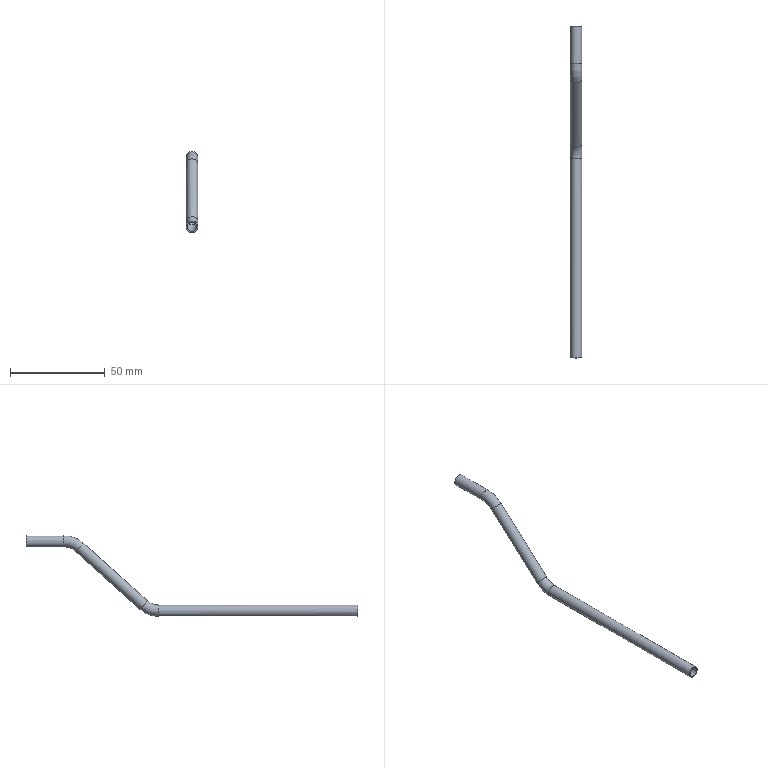Part | STEP file | 1-51.6 | 1 solid | 12 faces | box 6 x 175 x 42.678 mm | volume 1626 mm3 | cylinder 6 | torus 4 | plane 2 | commonest cylinder face diameters 5 x3 6 x3
STEP:
#1=CARTESIAN_POINT('',(0.,0.,0.));
#2=DIRECTION('',(0.,0.,1.));
#3=DIRECTION('',(1.,0.,0.));
#4=AXIS2_PLACEMENT_3D('',#1,#2,#3);
#5=CARTESIAN_POINT('',(3.,0.,0.));
#6=VERTEX_POINT('',#5);
#7=CARTESIAN_POINT('',(0.,0.,0.));
#8=DIRECTION('',(0.,-1.,0.));
#9=DIRECTION('',(1.,0.,0.));
#10=AXIS2_PLACEMENT_3D('',#7,#8,#9);
#11=CIRCLE('',#10,3.);
#12=CARTESIAN_POINT('',(0.,0.,0.));
#13=DIRECTION('',(0.,1.,0.));
#14=DIRECTION('',(1.,0.,0.));
#15=AXIS2_PLACEMENT_3D('',#12,#13,#14);
#16=CYLINDRICAL_SURFACE('',#15,3.);
#17=CARTESIAN_POINT('',(6.283,0.));
#18=DIRECTION('',(-1.,0.));
#19=VECTOR('',#18,1.);
#20=LINE('',#17,#19);
#21=(GEOMETRIC_REPRESENTATION_CONTEXT(2)PARAMETRIC_REPRESENTATION_CONTEXT()REPRESENTATION_CONTEXT('',''));
#22=DEFINITIONAL_REPRESENTATION('',(#20),#21);
#23=PCURVE('',#16,#22);
#24=CARTESIAN_POINT('',(0.,0.,0.));
#25=DIRECTION('',(0.,-1.,0.));
#26=DIRECTION('',(0.,0.,-1.));
#27=AXIS2_PLACEMENT_3D('',#24,#25,#26);
#28=PLANE('',#27);
#29=CARTESIAN_POINT('',(0.,0.));
#30=DIRECTION('',(0.,1.));
#31=AXIS2_PLACEMENT_2D('',#29,#30);
#32=CIRCLE('',#31,3.);
#33=(GEOMETRIC_REPRESENTATION_CONTEXT(2)PARAMETRIC_REPRESENTATION_CONTEXT()REPRESENTATION_CONTEXT('',''));
#34=DEFINITIONAL_REPRESENTATION('',(#32),#33);
#35=PCURVE('',#28,#34);
#36=SURFACE_CURVE('',#11,(#23,#35),.PCURVE_S1.);
#37=EDGE_CURVE('',#6,#6,#36,.T.);
#38=ORIENTED_EDGE('',*,*,#37,.F.);
#39=CARTESIAN_POINT('',(3.,105.,0.));
#40=VERTEX_POINT('',#39);
#41=CARTESIAN_POINT('',(3.,0.,0.));
#42=DIRECTION('',(0.,1.,0.));
#43=VECTOR('',#42,1.);
#44=LINE('',#41,#43);
#45=CARTESIAN_POINT('',(6.283,0.));
#46=DIRECTION('',(0.,1.));
#47=VECTOR('',#46,1.);
#48=LINE('',#45,#47);
#49=(GEOMETRIC_REPRESENTATION_CONTEXT(2)PARAMETRIC_REPRESENTATION_CONTEXT()REPRESENTATION_CONTEXT('',''));
#50=DEFINITIONAL_REPRESENTATION('',(#48),#49);
#51=PCURVE('',#16,#50);
#52=CARTESIAN_POINT('',(0.,0.));
#53=DIRECTION('',(0.,1.));
#54=VECTOR('',#53,1.);
#55=LINE('',#52,#54);
#56=(GEOMETRIC_REPRESENTATION_CONTEXT(2)PARAMETRIC_REPRESENTATION_CONTEXT()REPRESENTATION_CONTEXT('',''));
#57=DEFINITIONAL_REPRESENTATION('',(#55),#56);
#58=PCURVE('',#16,#57);
#59=SEAM_CURVE('',#44,(#51,#58),.PCURVE_S1.);
#60=EDGE_CURVE('',#6,#40,#59,.T.);
#61=ORIENTED_EDGE('',*,*,#60,.T.);
#62=CARTESIAN_POINT('',(0.,105.,-3.));
#63=VERTEX_POINT('',#62);
#64=CARTESIAN_POINT('',(0.,105.,0.));
#65=DIRECTION('',(0.,1.,0.));
#66=DIRECTION('',(0.,0.,-1.));
#67=AXIS2_PLACEMENT_3D('',#64,#65,#66);
#68=CIRCLE('',#67,3.);
#69=CARTESIAN_POINT('',(1.571,105.));
#70=DIRECTION('',(1.,0.));
#71=VECTOR('',#70,1.);
#72=LINE('',#69,#71);
#73=(GEOMETRIC_REPRESENTATION_CONTEXT(2)PARAMETRIC_REPRESENTATION_CONTEXT()REPRESENTATION_CONTEXT('',''));
#74=DEFINITIONAL_REPRESENTATION('',(#72),#73);
#75=PCURVE('',#16,#74);
#76=CARTESIAN_POINT('',(0.,105.,12.));
#77=DIRECTION('',(-1.,0.,0.));
#78=DIRECTION('',(0.,0.,-1.));
#79=AXIS2_PLACEMENT_3D('',#76,#77,#78);
#80=TOROIDAL_SURFACE('',#79,12.,3.);
#81=CARTESIAN_POINT('',(6.283,0.));
#82=DIRECTION('',(0.,1.));
#83=VECTOR('',#82,1.);
#84=LINE('',#81,#83);
#85=(GEOMETRIC_REPRESENTATION_CONTEXT(2)PARAMETRIC_REPRESENTATION_CONTEXT()REPRESENTATION_CONTEXT('',''));
#86=DEFINITIONAL_REPRESENTATION('',(#84),#85);
#87=PCURVE('',#80,#86);
#88=SURFACE_CURVE('',#68,(#75,#87),.PCURVE_S1.);
#89=EDGE_CURVE('',#63,#40,#88,.T.);
#90=ORIENTED_EDGE('',*,*,#89,.F.);
#91=CARTESIAN_POINT('',(0.,105.,0.));
#92=DIRECTION('',(0.,1.,0.));
#93=DIRECTION('',(1.,0.,0.));
#94=AXIS2_PLACEMENT_3D('',#91,#92,#93);
#95=CIRCLE('',#94,3.);
#96=CARTESIAN_POINT('',(0.,105.));
#97=DIRECTION('',(1.,0.));
#98=VECTOR('',#97,1.);
#99=LINE('',#96,#98);
#100=(GEOMETRIC_REPRESENTATION_CONTEXT(2)PARAMETRIC_REPRESENTATION_CONTEXT()REPRESENTATION_CONTEXT('',''));
#101=DEFINITIONAL_REPRESENTATION('',(#99),#100);
#102=PCURVE('',#16,#101);
#103=CARTESIAN_POINT('',(6.283,4.712));
#104=DIRECTION('',(0.,1.));
#105=VECTOR('',#104,1.);
#106=LINE('',#103,#105);
#107=(GEOMETRIC_REPRESENTATION_CONTEXT(2)PARAMETRIC_REPRESENTATION_CONTEXT()REPRESENTATION_CONTEXT('',''));
#108=DEFINITIONAL_REPRESENTATION('',(#106),#107);
#109=PCURVE('',#80,#108);
#110=SURFACE_CURVE('',#95,(#102,#109),.PCURVE_S1.);
#111=EDGE_CURVE('',#40,#63,#110,.T.);
#112=ORIENTED_EDGE('',*,*,#111,.F.);
#113=ORIENTED_EDGE('',*,*,#60,.F.);
#114=EDGE_LOOP('',(#38,#61,#90,#112,#113));
#115=FACE_BOUND('',#114,.T.);
#116=ADVANCED_FACE('',(#115),#16,.T.);
#117=ORIENTED_EDGE('',*,*,#89,.T.);
#118=ORIENTED_EDGE('',*,*,#111,.T.);
#119=CARTESIAN_POINT('',(0.,115.028,0.8451));
#120=VERTEX_POINT('',#119);
#121=CARTESIAN_POINT('',(0.,105.,12.));
#122=DIRECTION('',(1.,0.,0.));
#123=DIRECTION('',(0.,0.,-1.));
#124=AXIS2_PLACEMENT_3D('',#121,#122,#123);
#125=CIRCLE('',#124,15.);
#126=CARTESIAN_POINT('',(6.283,6.283));
#127=DIRECTION('',(-1.,0.));
#128=VECTOR('',#127,1.);
#129=LINE('',#126,#128);
#130=(GEOMETRIC_REPRESENTATION_CONTEXT(2)PARAMETRIC_REPRESENTATION_CONTEXT()REPRESENTATION_CONTEXT('',''));
#131=DEFINITIONAL_REPRESENTATION('',(#129),#130);
#132=PCURVE('',#80,#131);
#133=CARTESIAN_POINT('',(6.283,0.));
#134=DIRECTION('',(-1.,0.));
#135=VECTOR('',#134,1.);
#136=LINE('',#133,#135);
#137=(GEOMETRIC_REPRESENTATION_CONTEXT(2)PARAMETRIC_REPRESENTATION_CONTEXT()REPRESENTATION_CONTEXT('',''));
#138=DEFINITIONAL_REPRESENTATION('',(#136),#137);
#139=PCURVE('',#80,#138);
#140=SEAM_CURVE('',#125,(#132,#139),.PCURVE_S1.);
#141=EDGE_CURVE('',#63,#120,#140,.T.);
#142=ORIENTED_EDGE('',*,*,#141,.T.);
#143=CARTESIAN_POINT('',(3.,113.023,3.076));
#144=VERTEX_POINT('',#143);
#145=CARTESIAN_POINT('',(0.,113.023,3.076));
#146=DIRECTION('',(0.,-0.7437,-0.6686));
#147=DIRECTION('',(0.,0.6686,-0.7437));
#148=AXIS2_PLACEMENT_3D('',#145,#146,#147);
#149=CIRCLE('',#148,3.);
#150=CARTESIAN_POINT('',(5.551,6.283));
#151=DIRECTION('',(0.,-1.));
#152=VECTOR('',#151,1.);
#153=LINE('',#150,#152);
#154=(GEOMETRIC_REPRESENTATION_CONTEXT(2)PARAMETRIC_REPRESENTATION_CONTEXT()REPRESENTATION_CONTEXT('',''));
#155=DEFINITIONAL_REPRESENTATION('',(#153),#154);
#156=PCURVE('',#80,#155);
#157=CARTESIAN_POINT('',(0.,113.023,3.076));
#158=DIRECTION('',(0.,0.7437,0.6686));
#159=DIRECTION('',(1.,0.,0.));
#160=AXIS2_PLACEMENT_3D('',#157,#158,#159);
#161=CYLINDRICAL_SURFACE('',#160,3.);
#162=CARTESIAN_POINT('',(1.571,0.));
#163=DIRECTION('',(-1.,0.));
#164=VECTOR('',#163,1.);
#165=LINE('',#162,#164);
#166=(GEOMETRIC_REPRESENTATION_CONTEXT(2)PARAMETRIC_REPRESENTATION_CONTEXT()REPRESENTATION_CONTEXT('',''));
#167=DEFINITIONAL_REPRESENTATION('',(#165),#166);
#168=PCURVE('',#161,#167);
#169=SURFACE_CURVE('',#149,(#156,#168),.PCURVE_S1.);
#170=EDGE_CURVE('',#120,#144,#169,.T.);
#171=ORIENTED_EDGE('',*,*,#170,.T.);
#172=CARTESIAN_POINT('',(0.,113.023,3.076));
#173=DIRECTION('',(0.,-0.7437,-0.6686));
#174=DIRECTION('',(1.,0.,0.));
#175=AXIS2_PLACEMENT_3D('',#172,#173,#174);
#176=CIRCLE('',#175,3.);
#177=CARTESIAN_POINT('',(5.551,4.712));
#178=DIRECTION('',(0.,-1.));
#179=VECTOR('',#178,1.);
#180=LINE('',#177,#179);
#181=(GEOMETRIC_REPRESENTATION_CONTEXT(2)PARAMETRIC_REPRESENTATION_CONTEXT()REPRESENTATION_CONTEXT('',''));
#182=DEFINITIONAL_REPRESENTATION('',(#180),#181);
#183=PCURVE('',#80,#182);
#184=CARTESIAN_POINT('',(6.283,0.));
#185=DIRECTION('',(-1.,0.));
#186=VECTOR('',#185,1.);
#187=LINE('',#184,#186);
#188=(GEOMETRIC_REPRESENTATION_CONTEXT(2)PARAMETRIC_REPRESENTATION_CONTEXT()REPRESENTATION_CONTEXT('',''));
#189=DEFINITIONAL_REPRESENTATION('',(#187),#188);
#190=PCURVE('',#161,#189);
#191=SURFACE_CURVE('',#176,(#183,#190),.PCURVE_S1.);
#192=EDGE_CURVE('',#144,#120,#191,.T.);
#193=ORIENTED_EDGE('',*,*,#192,.T.);
#194=ORIENTED_EDGE('',*,*,#141,.F.);
#195=EDGE_LOOP('',(#117,#118,#142,#171,#193,#194));
#196=FACE_BOUND('',#195,.T.);
#197=ADVANCED_FACE('',(#196),#80,.T.);
#198=ORIENTED_EDGE('',*,*,#170,.F.);
#199=ORIENTED_EDGE('',*,*,#192,.F.);
#200=CARTESIAN_POINT('',(3.,146.977,33.602));
#201=VERTEX_POINT('',#200);
#202=CARTESIAN_POINT('',(3.,113.023,3.076));
#203=DIRECTION('',(0.,0.7437,0.6686));
#204=VECTOR('',#203,1.);
#205=LINE('',#202,#204);
#206=CARTESIAN_POINT('',(6.283,0.));
#207=DIRECTION('',(0.,1.));
#208=VECTOR('',#207,1.);
#209=LINE('',#206,#208);
#210=(GEOMETRIC_REPRESENTATION_CONTEXT(2)PARAMETRIC_REPRESENTATION_CONTEXT()REPRESENTATION_CONTEXT('',''));
#211=DEFINITIONAL_REPRESENTATION('',(#209),#210);
#212=PCURVE('',#161,#211);
#213=CARTESIAN_POINT('',(0.,0.));
#214=DIRECTION('',(0.,1.));
#215=VECTOR('',#214,1.);
#216=LINE('',#213,#215);
#217=(GEOMETRIC_REPRESENTATION_CONTEXT(2)PARAMETRIC_REPRESENTATION_CONTEXT()REPRESENTATION_CONTEXT('',''));
#218=DEFINITIONAL_REPRESENTATION('',(#216),#217);
#219=PCURVE('',#161,#218);
#220=SEAM_CURVE('',#205,(#212,#219),.PCURVE_S1.);
#221=EDGE_CURVE('',#144,#201,#220,.T.);
#222=ORIENTED_EDGE('',*,*,#221,.T.);
#223=CARTESIAN_POINT('',(-3.,146.977,33.602));
#224=VERTEX_POINT('',#223);
#225=CARTESIAN_POINT('',(0.,146.977,33.602));
#226=DIRECTION('',(0.,0.7437,0.6686));
#227=DIRECTION('',(-1.,0.,0.));
#228=AXIS2_PLACEMENT_3D('',#225,#226,#227);
#229=CIRCLE('',#228,3.);
#230=CARTESIAN_POINT('',(3.142,45.659));
#231=DIRECTION('',(1.,0.));
#232=VECTOR('',#231,1.);
#233=LINE('',#230,#232);
#234=(GEOMETRIC_REPRESENTATION_CONTEXT(2)PARAMETRIC_REPRESENTATION_CONTEXT()REPRESENTATION_CONTEXT('',''));
#235=DEFINITIONAL_REPRESENTATION('',(#233),#234);
#236=PCURVE('',#161,#235);
#237=CARTESIAN_POINT('',(0.,155.,24.678));
#238=DIRECTION('',(1.,0.,0.));
#239=DIRECTION('',(0.,-0.6686,0.7437));
#240=AXIS2_PLACEMENT_3D('',#237,#238,#239);
#241=TOROIDAL_SURFACE('',#240,12.,3.);
#242=CARTESIAN_POINT('',(6.283,-1.571));
#243=DIRECTION('',(0.,1.));
#244=VECTOR('',#243,1.);
#245=LINE('',#242,#244);
#246=(GEOMETRIC_REPRESENTATION_CONTEXT(2)PARAMETRIC_REPRESENTATION_CONTEXT()REPRESENTATION_CONTEXT('',''));
#247=DEFINITIONAL_REPRESENTATION('',(#245),#246);
#248=PCURVE('',#241,#247);
#249=SURFACE_CURVE('',#229,(#236,#248),.PCURVE_S1.);
#250=EDGE_CURVE('',#224,#201,#249,.T.);
#251=ORIENTED_EDGE('',*,*,#250,.F.);
#252=CARTESIAN_POINT('',(0.,146.977,33.602));
#253=DIRECTION('',(0.,0.7437,0.6686));
#254=DIRECTION('',(1.,0.,0.));
#255=AXIS2_PLACEMENT_3D('',#252,#253,#254);
#256=CIRCLE('',#255,3.);
#257=CARTESIAN_POINT('',(0.,45.659));
#258=DIRECTION('',(1.,0.));
#259=VECTOR('',#258,1.);
#260=LINE('',#257,#259);
#261=(GEOMETRIC_REPRESENTATION_CONTEXT(2)PARAMETRIC_REPRESENTATION_CONTEXT()REPRESENTATION_CONTEXT('',''));
#262=DEFINITIONAL_REPRESENTATION('',(#260),#261);
#263=PCURVE('',#161,#262);
#264=CARTESIAN_POINT('',(6.283,1.571));
#265=DIRECTION('',(0.,1.));
#266=VECTOR('',#265,1.);
#267=LINE('',#264,#266);
#268=(GEOMETRIC_REPRESENTATION_CONTEXT(2)PARAMETRIC_REPRESENTATION_CONTEXT()REPRESENTATION_CONTEXT('',''));
#269=DEFINITIONAL_REPRESENTATION('',(#267),#268);
#270=PCURVE('',#241,#269);
#271=SURFACE_CURVE('',#256,(#263,#270),.PCURVE_S1.);
#272=EDGE_CURVE('',#201,#224,#271,.T.);
#273=ORIENTED_EDGE('',*,*,#272,.F.);
#274=ORIENTED_EDGE('',*,*,#221,.F.);
#275=EDGE_LOOP('',(#198,#199,#222,#251,#273,#274));
#276=FACE_BOUND('',#275,.T.);
#277=ADVANCED_FACE('',(#276),#161,.T.);
#278=ORIENTED_EDGE('',*,*,#250,.T.);
#279=ORIENTED_EDGE('',*,*,#272,.T.);
#280=CARTESIAN_POINT('',(-3.,155.,36.678));
#281=VERTEX_POINT('',#280);
#282=CARTESIAN_POINT('',(-3.,155.,24.678));
#283=DIRECTION('',(-1.,0.,0.));
#284=DIRECTION('',(0.,-0.6686,0.7437));
#285=AXIS2_PLACEMENT_3D('',#282,#283,#284);
#286=CIRCLE('',#285,12.);
#287=CARTESIAN_POINT('',(6.283,4.712));
#288=DIRECTION('',(-1.,0.));
#289=VECTOR('',#288,1.);
#290=LINE('',#287,#289);
#291=(GEOMETRIC_REPRESENTATION_CONTEXT(2)PARAMETRIC_REPRESENTATION_CONTEXT()REPRESENTATION_CONTEXT('',''));
#292=DEFINITIONAL_REPRESENTATION('',(#290),#291);
#293=PCURVE('',#241,#292);
#294=CARTESIAN_POINT('',(6.283,-1.571));
#295=DIRECTION('',(-1.,0.));
#296=VECTOR('',#295,1.);
#297=LINE('',#294,#296);
#298=(GEOMETRIC_REPRESENTATION_CONTEXT(2)PARAMETRIC_REPRESENTATION_CONTEXT()REPRESENTATION_CONTEXT('',''));
#299=DEFINITIONAL_REPRESENTATION('',(#297),#298);
#300=PCURVE('',#241,#299);
#301=SEAM_CURVE('',#286,(#293,#300),.PCURVE_S1.);
#302=EDGE_CURVE('',#224,#281,#301,.T.);
#303=ORIENTED_EDGE('',*,*,#302,.T.);
#304=CARTESIAN_POINT('',(3.,155.,36.678));
#305=VERTEX_POINT('',#304);
#306=CARTESIAN_POINT('',(0.,155.,36.678));
#307=DIRECTION('',(0.,-1.,0.));
#308=DIRECTION('',(-1.,0.,0.));
#309=AXIS2_PLACEMENT_3D('',#306,#307,#308);
#310=CIRCLE('',#309,3.);
#311=CARTESIAN_POINT('',(5.551,4.712));
#312=DIRECTION('',(0.,-1.));
#313=VECTOR('',#312,1.);
#314=LINE('',#311,#313);
#315=(GEOMETRIC_REPRESENTATION_CONTEXT(2)PARAMETRIC_REPRESENTATION_CONTEXT()REPRESENTATION_CONTEXT('',''));
#316=DEFINITIONAL_REPRESENTATION('',(#314),#315);
#317=PCURVE('',#241,#316);
#318=CARTESIAN_POINT('',(0.,155.,36.678));
#319=DIRECTION('',(0.,1.,0.));
#320=DIRECTION('',(1.,0.,0.));
#321=AXIS2_PLACEMENT_3D('',#318,#319,#320);
#322=CYLINDRICAL_SURFACE('',#321,3.);
#323=CARTESIAN_POINT('',(3.142,0.));
#324=DIRECTION('',(-1.,0.));
#325=VECTOR('',#324,1.);
#326=LINE('',#323,#325);
#327=(GEOMETRIC_REPRESENTATION_CONTEXT(2)PARAMETRIC_REPRESENTATION_CONTEXT()REPRESENTATION_CONTEXT('',''));
#328=DEFINITIONAL_REPRESENTATION('',(#326),#327);
#329=PCURVE('',#322,#328);
#330=SURFACE_CURVE('',#310,(#317,#329),.PCURVE_S1.);
#331=EDGE_CURVE('',#281,#305,#330,.T.);
#332=ORIENTED_EDGE('',*,*,#331,.T.);
#333=CARTESIAN_POINT('',(0.,155.,36.678));
#334=DIRECTION('',(0.,-1.,0.));
#335=DIRECTION('',(1.,0.,0.));
#336=AXIS2_PLACEMENT_3D('',#333,#334,#335);
#337=CIRCLE('',#336,3.);
#338=CARTESIAN_POINT('',(5.551,1.571));
#339=DIRECTION('',(0.,-1.));
#340=VECTOR('',#339,1.);
#341=LINE('',#338,#340);
#342=(GEOMETRIC_REPRESENTATION_CONTEXT(2)PARAMETRIC_REPRESENTATION_CONTEXT()REPRESENTATION_CONTEXT('',''));
#343=DEFINITIONAL_REPRESENTATION('',(#341),#342);
#344=PCURVE('',#241,#343);
#345=CARTESIAN_POINT('',(6.283,0.));
#346=DIRECTION('',(-1.,0.));
#347=VECTOR('',#346,1.);
#348=LINE('',#345,#347);
#349=(GEOMETRIC_REPRESENTATION_CONTEXT(2)PARAMETRIC_REPRESENTATION_CONTEXT()REPRESENTATION_CONTEXT('',''));
#350=DEFINITIONAL_REPRESENTATION('',(#348),#349);
#351=PCURVE('',#322,#350);
#352=SURFACE_CURVE('',#337,(#344,#351),.PCURVE_S1.);
#353=EDGE_CURVE('',#305,#281,#352,.T.);
#354=ORIENTED_EDGE('',*,*,#353,.T.);
#355=ORIENTED_EDGE('',*,*,#302,.F.);
#356=EDGE_LOOP('',(#278,#279,#303,#332,#354,#355));
#357=FACE_BOUND('',#356,.T.);
#358=ADVANCED_FACE('',(#357),#241,.T.);
#359=ORIENTED_EDGE('',*,*,#331,.F.);
#360=ORIENTED_EDGE('',*,*,#353,.F.);
#361=CARTESIAN_POINT('',(3.,175.,36.678));
#362=VERTEX_POINT('',#361);
#363=CARTESIAN_POINT('',(3.,155.,36.678));
#364=DIRECTION('',(0.,1.,0.));
#365=VECTOR('',#364,1.);
#366=LINE('',#363,#365);
#367=CARTESIAN_POINT('',(6.283,0.));
#368=DIRECTION('',(0.,1.));
#369=VECTOR('',#368,1.);
#370=LINE('',#367,#369);
#371=(GEOMETRIC_REPRESENTATION_CONTEXT(2)PARAMETRIC_REPRESENTATION_CONTEXT()REPRESENTATION_CONTEXT('',''));
#372=DEFINITIONAL_REPRESENTATION('',(#370),#371);
#373=PCURVE('',#322,#372);
#374=CARTESIAN_POINT('',(0.,0.));
#375=DIRECTION('',(0.,1.));
#376=VECTOR('',#375,1.);
#377=LINE('',#374,#376);
#378=(GEOMETRIC_REPRESENTATION_CONTEXT(2)PARAMETRIC_REPRESENTATION_CONTEXT()REPRESENTATION_CONTEXT('',''));
#379=DEFINITIONAL_REPRESENTATION('',(#377),#378);
#380=PCURVE('',#322,#379);
#381=SEAM_CURVE('',#366,(#373,#380),.PCURVE_S1.);
#382=EDGE_CURVE('',#305,#362,#381,.T.);
#383=ORIENTED_EDGE('',*,*,#382,.T.);
#384=CARTESIAN_POINT('',(0.,175.,36.678));
#385=DIRECTION('',(0.,1.,0.));
#386=DIRECTION('',(1.,0.,0.));
#387=AXIS2_PLACEMENT_3D('',#384,#385,#386);
#388=CIRCLE('',#387,3.);
#389=CARTESIAN_POINT('',(0.,20.));
#390=DIRECTION('',(1.,0.));
#391=VECTOR('',#390,1.);
#392=LINE('',#389,#391);
#393=(GEOMETRIC_REPRESENTATION_CONTEXT(2)PARAMETRIC_REPRESENTATION_CONTEXT()REPRESENTATION_CONTEXT('',''));
#394=DEFINITIONAL_REPRESENTATION('',(#392),#393);
#395=PCURVE('',#322,#394);
#396=CARTESIAN_POINT('',(0.,175.,36.678));
#397=DIRECTION('',(0.,1.,0.));
#398=DIRECTION('',(0.,0.,1.));
#399=AXIS2_PLACEMENT_3D('',#396,#397,#398);
#400=PLANE('',#399);
#401=CARTESIAN_POINT('',(0.,0.));
#402=DIRECTION('',(0.,1.));
#403=AXIS2_PLACEMENT_2D('',#401,#402);
#404=CIRCLE('',#403,3.);
#405=(GEOMETRIC_REPRESENTATION_CONTEXT(2)PARAMETRIC_REPRESENTATION_CONTEXT()REPRESENTATION_CONTEXT('',''));
#406=DEFINITIONAL_REPRESENTATION('',(#404),#405);
#407=PCURVE('',#400,#406);
#408=SURFACE_CURVE('',#388,(#395,#407),.PCURVE_S1.);
#409=EDGE_CURVE('',#362,#362,#408,.T.);
#410=ORIENTED_EDGE('',*,*,#409,.F.);
#411=ORIENTED_EDGE('',*,*,#382,.F.);
#412=EDGE_LOOP('',(#359,#360,#383,#410,#411));
#413=FACE_BOUND('',#412,.T.);
#414=ADVANCED_FACE('',(#413),#322,.T.);
#415=ORIENTED_EDGE('',*,*,#37,.T.);
#416=EDGE_LOOP('',(#415));
#417=FACE_BOUND('',#416,.T.);
#418=CARTESIAN_POINT('',(2.5,0.,0.));
#419=VERTEX_POINT('',#418);
#420=CARTESIAN_POINT('',(0.,0.,0.));
#421=DIRECTION('',(0.,-1.,0.));
#422=DIRECTION('',(1.,0.,0.));
#423=AXIS2_PLACEMENT_3D('',#420,#421,#422);
#424=CIRCLE('',#423,2.5);
#425=CARTESIAN_POINT('',(0.,0.));
#426=DIRECTION('',(0.,1.));
#427=AXIS2_PLACEMENT_2D('',#425,#426);
#428=CIRCLE('',#427,2.5);
#429=(GEOMETRIC_REPRESENTATION_CONTEXT(2)PARAMETRIC_REPRESENTATION_CONTEXT()REPRESENTATION_CONTEXT('',''));
#430=DEFINITIONAL_REPRESENTATION('',(#428),#429);
#431=PCURVE('',#28,#430);
#432=CARTESIAN_POINT('',(0.,0.,0.));
#433=DIRECTION('',(0.,1.,0.));
#434=DIRECTION('',(1.,0.,0.));
#435=AXIS2_PLACEMENT_3D('',#432,#433,#434);
#436=CYLINDRICAL_SURFACE('',#435,2.5);
#437=CARTESIAN_POINT('',(6.283,0.));
#438=DIRECTION('',(-1.,0.));
#439=VECTOR('',#438,1.);
#440=LINE('',#437,#439);
#441=(GEOMETRIC_REPRESENTATION_CONTEXT(2)PARAMETRIC_REPRESENTATION_CONTEXT()REPRESENTATION_CONTEXT('',''));
#442=DEFINITIONAL_REPRESENTATION('',(#440),#441);
#443=PCURVE('',#436,#442);
#444=SURFACE_CURVE('',#424,(#431,#443),.PCURVE_S1.);
#445=EDGE_CURVE('',#419,#419,#444,.T.);
#446=ORIENTED_EDGE('',*,*,#445,.F.);
#447=EDGE_LOOP('',(#446));
#448=FACE_BOUND('',#447,.T.);
#449=ADVANCED_FACE('',(#417,#448),#28,.T.);
#450=ORIENTED_EDGE('',*,*,#409,.T.);
#451=EDGE_LOOP('',(#450));
#452=FACE_BOUND('',#451,.T.);
#453=CARTESIAN_POINT('',(2.5,175.,36.678));
#454=VERTEX_POINT('',#453);
#455=CARTESIAN_POINT('',(0.,175.,36.678));
#456=DIRECTION('',(0.,1.,0.));
#457=DIRECTION('',(1.,0.,0.));
#458=AXIS2_PLACEMENT_3D('',#455,#456,#457);
#459=CIRCLE('',#458,2.5);
#460=CARTESIAN_POINT('',(0.,0.));
#461=DIRECTION('',(0.,1.));
#462=AXIS2_PLACEMENT_2D('',#460,#461);
#463=CIRCLE('',#462,2.5);
#464=(GEOMETRIC_REPRESENTATION_CONTEXT(2)PARAMETRIC_REPRESENTATION_CONTEXT()REPRESENTATION_CONTEXT('',''));
#465=DEFINITIONAL_REPRESENTATION('',(#463),#464);
#466=PCURVE('',#400,#465);
#467=CARTESIAN_POINT('',(0.,155.,36.678));
#468=DIRECTION('',(0.,1.,0.));
#469=DIRECTION('',(1.,0.,0.));
#470=AXIS2_PLACEMENT_3D('',#467,#468,#469);
#471=CYLINDRICAL_SURFACE('',#470,2.5);
#472=CARTESIAN_POINT('',(0.,20.));
#473=DIRECTION('',(1.,0.));
#474=VECTOR('',#473,1.);
#475=LINE('',#472,#474);
#476=(GEOMETRIC_REPRESENTATION_CONTEXT(2)PARAMETRIC_REPRESENTATION_CONTEXT()REPRESENTATION_CONTEXT('',''));
#477=DEFINITIONAL_REPRESENTATION('',(#475),#476);
#478=PCURVE('',#471,#477);
#479=SURFACE_CURVE('',#459,(#466,#478),.PCURVE_S1.);
#480=EDGE_CURVE('',#454,#454,#479,.T.);
#481=ORIENTED_EDGE('',*,*,#480,.F.);
#482=EDGE_LOOP('',(#481));
#483=FACE_BOUND('',#482,.T.);
#484=ADVANCED_FACE('',(#452,#483),#400,.T.);
#485=ORIENTED_EDGE('',*,*,#445,.F.);
#486=CARTESIAN_POINT('',(2.5,105.,0.));
#487=VERTEX_POINT('',#486);
#488=CARTESIAN_POINT('',(2.5,0.,0.));
#489=DIRECTION('',(0.,1.,0.));
#490=VECTOR('',#489,1.);
#491=LINE('',#488,#490);
#492=CARTESIAN_POINT('',(6.283,0.));
#493=DIRECTION('',(0.,1.));
#494=VECTOR('',#493,1.);
#495=LINE('',#492,#494);
#496=(GEOMETRIC_REPRESENTATION_CONTEXT(2)PARAMETRIC_REPRESENTATION_CONTEXT()REPRESENTATION_CONTEXT('',''));
#497=DEFINITIONAL_REPRESENTATION('',(#495),#496);
#498=PCURVE('',#436,#497);
#499=CARTESIAN_POINT('',(0.,0.));
#500=DIRECTION('',(0.,1.));
#501=VECTOR('',#500,1.);
#502=LINE('',#499,#501);
#503=(GEOMETRIC_REPRESENTATION_CONTEXT(2)PARAMETRIC_REPRESENTATION_CONTEXT()REPRESENTATION_CONTEXT('',''));
#504=DEFINITIONAL_REPRESENTATION('',(#502),#503);
#505=PCURVE('',#436,#504);
#506=SEAM_CURVE('',#491,(#498,#505),.PCURVE_S1.);
#507=EDGE_CURVE('',#419,#487,#506,.T.);
#508=ORIENTED_EDGE('',*,*,#507,.T.);
#509=CARTESIAN_POINT('',(0.,105.,-2.5));
#510=VERTEX_POINT('',#509);
#511=CARTESIAN_POINT('',(0.,105.,0.));
#512=DIRECTION('',(0.,1.,0.));
#513=DIRECTION('',(0.,0.,-1.));
#514=AXIS2_PLACEMENT_3D('',#511,#512,#513);
#515=CIRCLE('',#514,2.5);
#516=CARTESIAN_POINT('',(1.571,105.));
#517=DIRECTION('',(1.,0.));
#518=VECTOR('',#517,1.);
#519=LINE('',#516,#518);
#520=(GEOMETRIC_REPRESENTATION_CONTEXT(2)PARAMETRIC_REPRESENTATION_CONTEXT()REPRESENTATION_CONTEXT('',''));
#521=DEFINITIONAL_REPRESENTATION('',(#519),#520);
#522=PCURVE('',#436,#521);
#523=CARTESIAN_POINT('',(0.,105.,12.));
#524=DIRECTION('',(-1.,0.,0.));
#525=DIRECTION('',(0.,0.,-1.));
#526=AXIS2_PLACEMENT_3D('',#523,#524,#525);
#527=TOROIDAL_SURFACE('',#526,12.,2.5);
#528=CARTESIAN_POINT('',(6.283,0.));
#529=CARTESIAN_POINT('',(6.283,0.0714));
#530=CARTESIAN_POINT('',(6.283,0.2142));
#531=CARTESIAN_POINT('',(6.283,0.4284));
#532=CARTESIAN_POINT('',(6.283,0.6426));
#533=CARTESIAN_POINT('',(6.283,0.8568));
#534=CARTESIAN_POINT('',(6.283,1.071));
#535=CARTESIAN_POINT('',(6.283,1.285));
#536=CARTESIAN_POINT('',(6.283,1.499));
#537=CARTESIAN_POINT('',(6.283,1.714));
#538=CARTESIAN_POINT('',(6.283,1.928));
#539=CARTESIAN_POINT('',(6.283,2.142));
#540=CARTESIAN_POINT('',(6.283,2.356));
#541=CARTESIAN_POINT('',(6.283,2.57));
#542=CARTESIAN_POINT('',(6.283,2.785));
#543=CARTESIAN_POINT('',(6.283,2.999));
#544=CARTESIAN_POINT('',(6.283,3.213));
#545=CARTESIAN_POINT('',(6.283,3.427));
#546=CARTESIAN_POINT('',(6.283,3.641));
#547=CARTESIAN_POINT('',(6.283,3.856));
#548=CARTESIAN_POINT('',(6.283,4.07));
#549=CARTESIAN_POINT('',(6.283,4.284));
#550=CARTESIAN_POINT('',(6.283,4.498));
#551=CARTESIAN_POINT('',(6.283,4.641));
#552=CARTESIAN_POINT('',(6.283,4.712));
#553=B_SPLINE_CURVE_WITH_KNOTS('',3,(#528,#529,#530,#531,#532,#533,#534,#535,#536,#537,#538,#539,#540,#541,#542,#543,#544,#545,#546,#547,#548,#549,#550,#551,#552),.UNSPECIFIED.,.F.,.F.,(4,1,1,1,1,1,1,1,1,1,1,1,1,1,1,1,1,1,1,1,1,1,4),(0.,0.2142,0.4284,0.6426,0.8568,1.071,1.285,1.499,1.714,1.928,2.142,2.356,2.57,2.785,2.999,3.213,3.427,3.641,3.856,4.07,4.284,4.498,4.712),.QUASI_UNIFORM_KNOTS.);
#554=(GEOMETRIC_REPRESENTATION_CONTEXT(2)PARAMETRIC_REPRESENTATION_CONTEXT()REPRESENTATION_CONTEXT('',''));
#555=DEFINITIONAL_REPRESENTATION('',(#553),#554);
#556=PCURVE('',#527,#555);
#557=SURFACE_CURVE('',#515,(#522,#556),.PCURVE_S1.);
#558=EDGE_CURVE('',#510,#487,#557,.T.);
#559=ORIENTED_EDGE('',*,*,#558,.F.);
#560=CARTESIAN_POINT('',(0.,105.,0.));
#561=DIRECTION('',(0.,1.,0.));
#562=DIRECTION('',(1.,0.,0.));
#563=AXIS2_PLACEMENT_3D('',#560,#561,#562);
#564=CIRCLE('',#563,2.5);
#565=CARTESIAN_POINT('',(0.,105.));
#566=DIRECTION('',(1.,0.));
#567=VECTOR('',#566,1.);
#568=LINE('',#565,#567);
#569=(GEOMETRIC_REPRESENTATION_CONTEXT(2)PARAMETRIC_REPRESENTATION_CONTEXT()REPRESENTATION_CONTEXT('',''));
#570=DEFINITIONAL_REPRESENTATION('',(#568),#569);
#571=PCURVE('',#436,#570);
#572=CARTESIAN_POINT('',(6.283,4.712));
#573=DIRECTION('',(0.,1.));
#574=VECTOR('',#573,1.);
#575=LINE('',#572,#574);
#576=(GEOMETRIC_REPRESENTATION_CONTEXT(2)PARAMETRIC_REPRESENTATION_CONTEXT()REPRESENTATION_CONTEXT('',''));
#577=DEFINITIONAL_REPRESENTATION('',(#575),#576);
#578=PCURVE('',#527,#577);
#579=SURFACE_CURVE('',#564,(#571,#578),.PCURVE_S1.);
#580=EDGE_CURVE('',#487,#510,#579,.T.);
#581=ORIENTED_EDGE('',*,*,#580,.F.);
#582=ORIENTED_EDGE('',*,*,#507,.F.);
#583=EDGE_LOOP('',(#485,#508,#559,#581,#582));
#584=FACE_BOUND('',#583,.F.);
#585=ADVANCED_FACE('',(#584),#436,.F.);
#586=ORIENTED_EDGE('',*,*,#558,.T.);
#587=ORIENTED_EDGE('',*,*,#580,.T.);
#588=CARTESIAN_POINT('',(0.,114.694,1.217));
#589=VERTEX_POINT('',#588);
#590=CARTESIAN_POINT('',(0.,105.,12.));
#591=DIRECTION('',(1.,0.,0.));
#592=DIRECTION('',(0.,0.,-1.));
#593=AXIS2_PLACEMENT_3D('',#590,#591,#592);
#594=CIRCLE('',#593,14.5);
#595=CARTESIAN_POINT('',(6.283,6.283));
#596=DIRECTION('',(-1.,0.));
#597=VECTOR('',#596,1.);
#598=LINE('',#595,#597);
#599=(GEOMETRIC_REPRESENTATION_CONTEXT(2)PARAMETRIC_REPRESENTATION_CONTEXT()REPRESENTATION_CONTEXT('',''));
#600=DEFINITIONAL_REPRESENTATION('',(#598),#599);
#601=PCURVE('',#527,#600);
#602=CARTESIAN_POINT('',(6.283,0.));
#603=DIRECTION('',(-1.,0.));
#604=VECTOR('',#603,1.);
#605=LINE('',#602,#604);
#606=(GEOMETRIC_REPRESENTATION_CONTEXT(2)PARAMETRIC_REPRESENTATION_CONTEXT()REPRESENTATION_CONTEXT('',''));
#607=DEFINITIONAL_REPRESENTATION('',(#605),#606);
#608=PCURVE('',#527,#607);
#609=SEAM_CURVE('',#594,(#601,#608),.PCURVE_S1.);
#610=EDGE_CURVE('',#510,#589,#609,.T.);
#611=ORIENTED_EDGE('',*,*,#610,.T.);
#612=CARTESIAN_POINT('',(2.5,113.023,3.076));
#613=VERTEX_POINT('',#612);
#614=CARTESIAN_POINT('',(0.,113.023,3.076));
#615=DIRECTION('',(0.,-0.7437,-0.6686));
#616=DIRECTION('',(0.,0.6686,-0.7437));
#617=AXIS2_PLACEMENT_3D('',#614,#615,#616);
#618=CIRCLE('',#617,2.5);
#619=CARTESIAN_POINT('',(5.551,6.283));
#620=DIRECTION('',(0.,-1.));
#621=VECTOR('',#620,1.);
#622=LINE('',#619,#621);
#623=(GEOMETRIC_REPRESENTATION_CONTEXT(2)PARAMETRIC_REPRESENTATION_CONTEXT()REPRESENTATION_CONTEXT('',''));
#624=DEFINITIONAL_REPRESENTATION('',(#622),#623);
#625=PCURVE('',#527,#624);
#626=CARTESIAN_POINT('',(0.,113.023,3.076));
#627=DIRECTION('',(0.,0.7437,0.6686));
#628=DIRECTION('',(1.,0.,0.));
#629=AXIS2_PLACEMENT_3D('',#626,#627,#628);
#630=CYLINDRICAL_SURFACE('',#629,2.5);
#631=CARTESIAN_POINT('',(1.571,0.));
#632=DIRECTION('',(-1.,0.));
#633=VECTOR('',#632,1.);
#634=LINE('',#631,#633);
#635=(GEOMETRIC_REPRESENTATION_CONTEXT(2)PARAMETRIC_REPRESENTATION_CONTEXT()REPRESENTATION_CONTEXT('',''));
#636=DEFINITIONAL_REPRESENTATION('',(#634),#635);
#637=PCURVE('',#630,#636);
#638=SURFACE_CURVE('',#618,(#625,#637),.PCURVE_S1.);
#639=EDGE_CURVE('',#589,#613,#638,.T.);
#640=ORIENTED_EDGE('',*,*,#639,.T.);
#641=CARTESIAN_POINT('',(0.,113.023,3.076));
#642=DIRECTION('',(0.,-0.7437,-0.6686));
#643=DIRECTION('',(1.,0.,0.));
#644=AXIS2_PLACEMENT_3D('',#641,#642,#643);
#645=CIRCLE('',#644,2.5);
#646=CARTESIAN_POINT('',(5.551,4.712));
#647=DIRECTION('',(0.,-1.));
#648=VECTOR('',#647,1.);
#649=LINE('',#646,#648);
#650=(GEOMETRIC_REPRESENTATION_CONTEXT(2)PARAMETRIC_REPRESENTATION_CONTEXT()REPRESENTATION_CONTEXT('',''));
#651=DEFINITIONAL_REPRESENTATION('',(#649),#650);
#652=PCURVE('',#527,#651);
#653=CARTESIAN_POINT('',(6.283,0.));
#654=DIRECTION('',(-1.,0.));
#655=VECTOR('',#654,1.);
#656=LINE('',#653,#655);
#657=(GEOMETRIC_REPRESENTATION_CONTEXT(2)PARAMETRIC_REPRESENTATION_CONTEXT()REPRESENTATION_CONTEXT('',''));
#658=DEFINITIONAL_REPRESENTATION('',(#656),#657);
#659=PCURVE('',#630,#658);
#660=SURFACE_CURVE('',#645,(#652,#659),.PCURVE_S1.);
#661=EDGE_CURVE('',#613,#589,#660,.T.);
#662=ORIENTED_EDGE('',*,*,#661,.T.);
#663=ORIENTED_EDGE('',*,*,#610,.F.);
#664=EDGE_LOOP('',(#586,#587,#611,#640,#662,#663));
#665=FACE_BOUND('',#664,.F.);
#666=ADVANCED_FACE('',(#665),#527,.F.);
#667=ORIENTED_EDGE('',*,*,#639,.F.);
#668=ORIENTED_EDGE('',*,*,#661,.F.);
#669=CARTESIAN_POINT('',(2.5,146.977,33.602));
#670=VERTEX_POINT('',#669);
#671=CARTESIAN_POINT('',(2.5,113.023,3.076));
#672=DIRECTION('',(0.,0.7437,0.6686));
#673=VECTOR('',#672,1.);
#674=LINE('',#671,#673);
#675=CARTESIAN_POINT('',(6.283,0.));
#676=DIRECTION('',(0.,1.));
#677=VECTOR('',#676,1.);
#678=LINE('',#675,#677);
#679=(GEOMETRIC_REPRESENTATION_CONTEXT(2)PARAMETRIC_REPRESENTATION_CONTEXT()REPRESENTATION_CONTEXT('',''));
#680=DEFINITIONAL_REPRESENTATION('',(#678),#679);
#681=PCURVE('',#630,#680);
#682=CARTESIAN_POINT('',(0.,0.));
#683=DIRECTION('',(0.,1.));
#684=VECTOR('',#683,1.);
#685=LINE('',#682,#684);
#686=(GEOMETRIC_REPRESENTATION_CONTEXT(2)PARAMETRIC_REPRESENTATION_CONTEXT()REPRESENTATION_CONTEXT('',''));
#687=DEFINITIONAL_REPRESENTATION('',(#685),#686);
#688=PCURVE('',#630,#687);
#689=SEAM_CURVE('',#674,(#681,#688),.PCURVE_S1.);
#690=EDGE_CURVE('',#613,#670,#689,.T.);
#691=ORIENTED_EDGE('',*,*,#690,.T.);
#692=CARTESIAN_POINT('',(-2.5,146.977,33.602));
#693=VERTEX_POINT('',#692);
#694=CARTESIAN_POINT('',(0.,146.977,33.602));
#695=DIRECTION('',(0.,0.7437,0.6686));
#696=DIRECTION('',(-1.,0.,0.));
#697=AXIS2_PLACEMENT_3D('',#694,#695,#696);
#698=CIRCLE('',#697,2.5);
#699=CARTESIAN_POINT('',(3.142,45.659));
#700=DIRECTION('',(1.,0.));
#701=VECTOR('',#700,1.);
#702=LINE('',#699,#701);
#703=(GEOMETRIC_REPRESENTATION_CONTEXT(2)PARAMETRIC_REPRESENTATION_CONTEXT()REPRESENTATION_CONTEXT('',''));
#704=DEFINITIONAL_REPRESENTATION('',(#702),#703);
#705=PCURVE('',#630,#704);
#706=CARTESIAN_POINT('',(0.,155.,24.678));
#707=DIRECTION('',(1.,0.,0.));
#708=DIRECTION('',(0.,-0.6686,0.7437));
#709=AXIS2_PLACEMENT_3D('',#706,#707,#708);
#710=TOROIDAL_SURFACE('',#709,12.,2.5);
#711=CARTESIAN_POINT('',(6.283,-1.571));
#712=DIRECTION('',(0.,1.));
#713=VECTOR('',#712,1.);
#714=LINE('',#711,#713);
#715=(GEOMETRIC_REPRESENTATION_CONTEXT(2)PARAMETRIC_REPRESENTATION_CONTEXT()REPRESENTATION_CONTEXT('',''));
#716=DEFINITIONAL_REPRESENTATION('',(#714),#715);
#717=PCURVE('',#710,#716);
#718=SURFACE_CURVE('',#698,(#705,#717),.PCURVE_S1.);
#719=EDGE_CURVE('',#693,#670,#718,.T.);
#720=ORIENTED_EDGE('',*,*,#719,.F.);
#721=CARTESIAN_POINT('',(0.,146.977,33.602));
#722=DIRECTION('',(0.,0.7437,0.6686));
#723=DIRECTION('',(1.,0.,0.));
#724=AXIS2_PLACEMENT_3D('',#721,#722,#723);
#725=CIRCLE('',#724,2.5);
#726=CARTESIAN_POINT('',(0.,45.659));
#727=DIRECTION('',(1.,0.));
#728=VECTOR('',#727,1.);
#729=LINE('',#726,#728);
#730=(GEOMETRIC_REPRESENTATION_CONTEXT(2)PARAMETRIC_REPRESENTATION_CONTEXT()REPRESENTATION_CONTEXT('',''));
#731=DEFINITIONAL_REPRESENTATION('',(#729),#730);
#732=PCURVE('',#630,#731);
#733=CARTESIAN_POINT('',(6.283,1.571));
#734=DIRECTION('',(0.,1.));
#735=VECTOR('',#734,1.);
#736=LINE('',#733,#735);
#737=(GEOMETRIC_REPRESENTATION_CONTEXT(2)PARAMETRIC_REPRESENTATION_CONTEXT()REPRESENTATION_CONTEXT('',''));
#738=DEFINITIONAL_REPRESENTATION('',(#736),#737);
#739=PCURVE('',#710,#738);
#740=SURFACE_CURVE('',#725,(#732,#739),.PCURVE_S1.);
#741=EDGE_CURVE('',#670,#693,#740,.T.);
#742=ORIENTED_EDGE('',*,*,#741,.F.);
#743=ORIENTED_EDGE('',*,*,#690,.F.);
#744=EDGE_LOOP('',(#667,#668,#691,#720,#742,#743));
#745=FACE_BOUND('',#744,.F.);
#746=ADVANCED_FACE('',(#745),#630,.F.);
#747=ORIENTED_EDGE('',*,*,#719,.T.);
#748=ORIENTED_EDGE('',*,*,#741,.T.);
#749=CARTESIAN_POINT('',(-2.5,155.,36.678));
#750=VERTEX_POINT('',#749);
#751=CARTESIAN_POINT('',(-2.5,155.,24.678));
#752=DIRECTION('',(-1.,0.,0.));
#753=DIRECTION('',(0.,-0.6686,0.7437));
#754=AXIS2_PLACEMENT_3D('',#751,#752,#753);
#755=CIRCLE('',#754,12.);
#756=CARTESIAN_POINT('',(6.283,4.712));
#757=DIRECTION('',(-1.,0.));
#758=VECTOR('',#757,1.);
#759=LINE('',#756,#758);
#760=(GEOMETRIC_REPRESENTATION_CONTEXT(2)PARAMETRIC_REPRESENTATION_CONTEXT()REPRESENTATION_CONTEXT('',''));
#761=DEFINITIONAL_REPRESENTATION('',(#759),#760);
#762=PCURVE('',#710,#761);
#763=CARTESIAN_POINT('',(6.283,-1.571));
#764=DIRECTION('',(-1.,0.));
#765=VECTOR('',#764,1.);
#766=LINE('',#763,#765);
#767=(GEOMETRIC_REPRESENTATION_CONTEXT(2)PARAMETRIC_REPRESENTATION_CONTEXT()REPRESENTATION_CONTEXT('',''));
#768=DEFINITIONAL_REPRESENTATION('',(#766),#767);
#769=PCURVE('',#710,#768);
#770=SEAM_CURVE('',#755,(#762,#769),.PCURVE_S1.);
#771=EDGE_CURVE('',#693,#750,#770,.T.);
#772=ORIENTED_EDGE('',*,*,#771,.T.);
#773=CARTESIAN_POINT('',(2.5,155.,36.678));
#774=VERTEX_POINT('',#773);
#775=CARTESIAN_POINT('',(0.,155.,36.678));
#776=DIRECTION('',(0.,-1.,0.));
#777=DIRECTION('',(-1.,0.,0.));
#778=AXIS2_PLACEMENT_3D('',#775,#776,#777);
#779=CIRCLE('',#778,2.5);
#780=CARTESIAN_POINT('',(5.551,4.712));
#781=DIRECTION('',(0.,-1.));
#782=VECTOR('',#781,1.);
#783=LINE('',#780,#782);
#784=(GEOMETRIC_REPRESENTATION_CONTEXT(2)PARAMETRIC_REPRESENTATION_CONTEXT()REPRESENTATION_CONTEXT('',''));
#785=DEFINITIONAL_REPRESENTATION('',(#783),#784);
#786=PCURVE('',#710,#785);
#787=CARTESIAN_POINT('',(3.142,0.));
#788=DIRECTION('',(-1.,0.));
#789=VECTOR('',#788,1.);
#790=LINE('',#787,#789);
#791=(GEOMETRIC_REPRESENTATION_CONTEXT(2)PARAMETRIC_REPRESENTATION_CONTEXT()REPRESENTATION_CONTEXT('',''));
#792=DEFINITIONAL_REPRESENTATION('',(#790),#791);
#793=PCURVE('',#471,#792);
#794=SURFACE_CURVE('',#779,(#786,#793),.PCURVE_S1.);
#795=EDGE_CURVE('',#750,#774,#794,.T.);
#796=ORIENTED_EDGE('',*,*,#795,.T.);
#797=CARTESIAN_POINT('',(0.,155.,36.678));
#798=DIRECTION('',(0.,-1.,0.));
#799=DIRECTION('',(1.,0.,0.));
#800=AXIS2_PLACEMENT_3D('',#797,#798,#799);
#801=CIRCLE('',#800,2.5);
#802=CARTESIAN_POINT('',(5.551,1.571));
#803=DIRECTION('',(0.,-1.));
#804=VECTOR('',#803,1.);
#805=LINE('',#802,#804);
#806=(GEOMETRIC_REPRESENTATION_CONTEXT(2)PARAMETRIC_REPRESENTATION_CONTEXT()REPRESENTATION_CONTEXT('',''));
#807=DEFINITIONAL_REPRESENTATION('',(#805),#806);
#808=PCURVE('',#710,#807);
#809=CARTESIAN_POINT('',(6.283,0.));
#810=DIRECTION('',(-1.,0.));
#811=VECTOR('',#810,1.);
#812=LINE('',#809,#811);
#813=(GEOMETRIC_REPRESENTATION_CONTEXT(2)PARAMETRIC_REPRESENTATION_CONTEXT()REPRESENTATION_CONTEXT('',''));
#814=DEFINITIONAL_REPRESENTATION('',(#812),#813);
#815=PCURVE('',#471,#814);
#816=SURFACE_CURVE('',#801,(#808,#815),.PCURVE_S1.);
#817=EDGE_CURVE('',#774,#750,#816,.T.);
#818=ORIENTED_EDGE('',*,*,#817,.T.);
#819=ORIENTED_EDGE('',*,*,#771,.F.);
#820=EDGE_LOOP('',(#747,#748,#772,#796,#818,#819));
#821=FACE_BOUND('',#820,.F.);
#822=ADVANCED_FACE('',(#821),#710,.F.);
#823=ORIENTED_EDGE('',*,*,#795,.F.);
#824=ORIENTED_EDGE('',*,*,#817,.F.);
#825=CARTESIAN_POINT('',(2.5,155.,36.678));
#826=DIRECTION('',(0.,1.,0.));
#827=VECTOR('',#826,1.);
#828=LINE('',#825,#827);
#829=CARTESIAN_POINT('',(6.283,0.));
#830=DIRECTION('',(0.,1.));
#831=VECTOR('',#830,1.);
#832=LINE('',#829,#831);
#833=(GEOMETRIC_REPRESENTATION_CONTEXT(2)PARAMETRIC_REPRESENTATION_CONTEXT()REPRESENTATION_CONTEXT('',''));
#834=DEFINITIONAL_REPRESENTATION('',(#832),#833);
#835=PCURVE('',#471,#834);
#836=CARTESIAN_POINT('',(0.,0.));
#837=DIRECTION('',(0.,1.));
#838=VECTOR('',#837,1.);
#839=LINE('',#836,#838);
#840=(GEOMETRIC_REPRESENTATION_CONTEXT(2)PARAMETRIC_REPRESENTATION_CONTEXT()REPRESENTATION_CONTEXT('',''));
#841=DEFINITIONAL_REPRESENTATION('',(#839),#840);
#842=PCURVE('',#471,#841);
#843=SEAM_CURVE('',#828,(#835,#842),.PCURVE_S1.);
#844=EDGE_CURVE('',#774,#454,#843,.T.);
#845=ORIENTED_EDGE('',*,*,#844,.T.);
#846=ORIENTED_EDGE('',*,*,#480,.F.);
#847=ORIENTED_EDGE('',*,*,#844,.F.);
#848=EDGE_LOOP('',(#823,#824,#845,#846,#847));
#849=FACE_BOUND('',#848,.F.);
#850=ADVANCED_FACE('',(#849),#471,.F.);
#851=CLOSED_SHELL('',(#116,#197,#277,#358,#414,#449,#484,#585,#666,#746,#822,#850));
#852=MANIFOLD_SOLID_BREP('',#851);
#853=(LENGTH_UNIT()NAMED_UNIT(*)SI_UNIT(.MILLI.,.METRE.));
#854=UNCERTAINTY_MEASURE_WITH_UNIT(LENGTH_MEASURE(0.0000001),#853,'','');
#855=(NAMED_UNIT(*)PLANE_ANGLE_UNIT()SI_UNIT($,.RADIAN.));
#856=(NAMED_UNIT(*)SI_UNIT($,.STERADIAN.)SOLID_ANGLE_UNIT());
#857=(GEOMETRIC_REPRESENTATION_CONTEXT(3)GLOBAL_UNCERTAINTY_ASSIGNED_CONTEXT((#854))GLOBAL_UNIT_ASSIGNED_CONTEXT((#853,#855,#856))REPRESENTATION_CONTEXT('',''));
#858=ADVANCED_BREP_SHAPE_REPRESENTATION('',(#4,#852),#857);